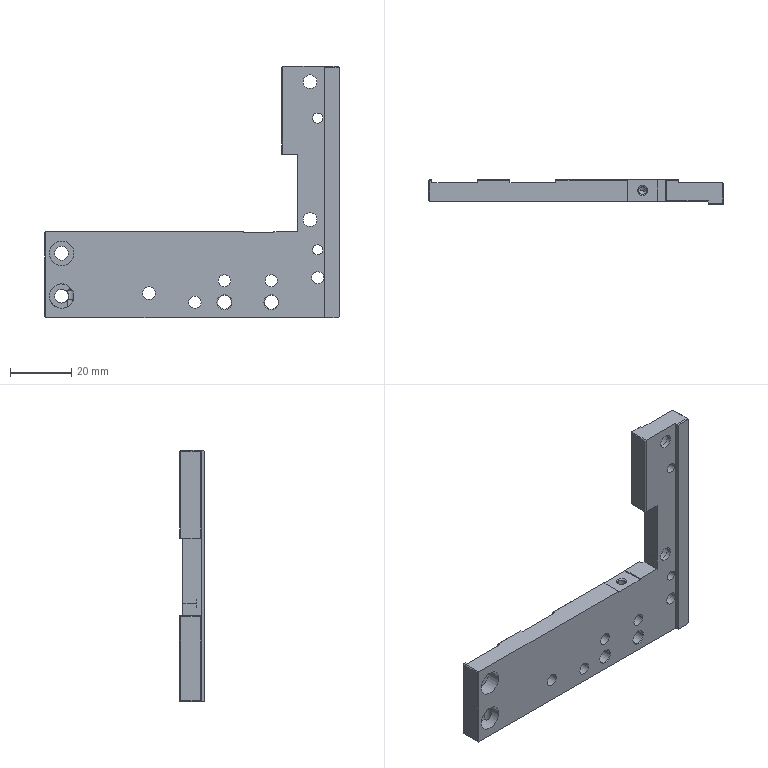Part | NX | 1 solid | 117 faces | box 96.1 x 8 x 82 mm | volume 21519 mm3 | plane 49 | cylinder 42 | cone 26 | commonest cylinder face diameters 4.5 x12 2.5 x8 4 x8 8 x8 3.3 x4 4.2 x2